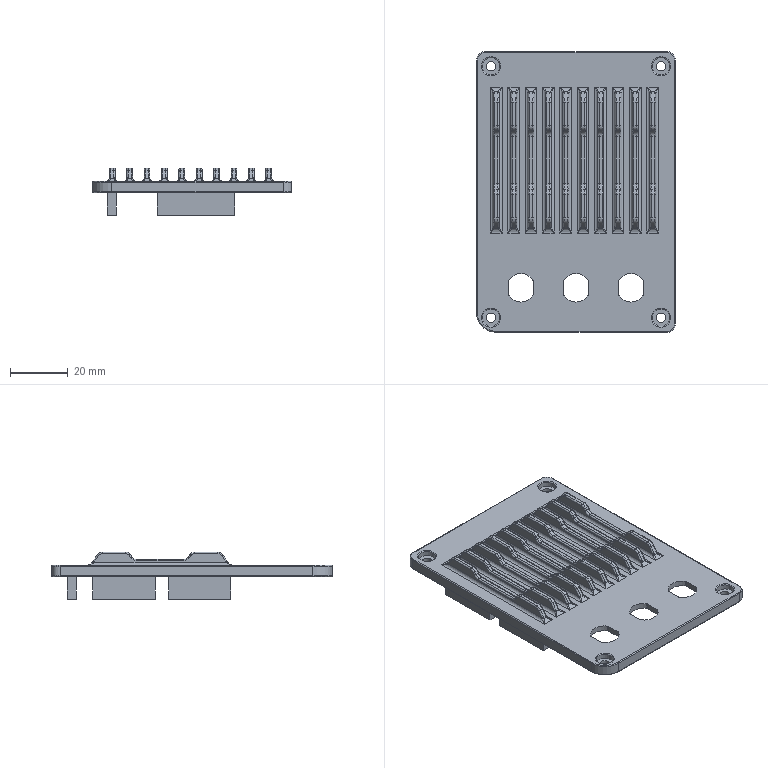NC program | NX | posted with a generic post | part box 68.665 x 96.782 x 16.5 mm
Lines 4650 to 4797 of 111885:
(PLANAR_MILL_COPY_1 , TOOL : 倒角刀)
N9238 T03 M6
N9240 G53
N9242 G17 G0 G90 X-41.991 Y-16.732 S4500 M3
N9244 G43 Z20. H3
N9246 Z2.
N9248 G94 G1 Z-1. F1000.
N9250 G3 X-42.991 Y-15.732 R1.
N9252 G2 X-43.991 Y-14.733 R1.
N9254 G1 X-44.009 Y12.049
N9256 G2 X-43.015 Y13.05 R1.
N9258 G1 X-39.897 Y13.068
N9260 G2 X-38.891 Y12.068 R1.
N9262 G1 Y-14.732
N9264 G2 X-39.891 Y-15.732 R1.
N9266 G1 X-42.991
N9268 G3 X-43.991 Y-16.732 R1.
N9270 G1 Z2.
N9272 G0 Z20.
N9274 X-10.709 Y27.168
N9276 Z2.
N9278 G1 Z-1.
N9280 G3 X-11.709 Y26.168 R1.
N9282 G2 X-12.709 Y25.168 R1.
N9284 G1 X-34.191
N9286 G2 X-35.191 Y26.168 R1.
N9288 G1 Y29.286
N9290 G2 X-34.191 Y30.286 R1.
N9292 G1 X-12.709
N9294 G2 X-11.709 Y29.286 R1.
N9296 G1 Y26.168
N9298 G3 X-10.709 Y25.168 R1.
N9300 G1 Z2.
N9302 G0 Z20.
N9304 X15.409 Y27.168
N9306 Z2.
N9308 G1 Z-1.
N9310 G3 X14.409 Y26.168 R1.
N9312 G2 X13.409 Y25.168 R1.
N9314 G1 X-8.073
N9316 G2 X-9.073 Y26.168 R1.
N9318 G1 Y29.286
N9320 G2 X-8.073 Y30.286 R1.
N9322 G1 X13.409
N9324 G2 X14.409 Y29.286 R1.
N9326 G1 Y26.168
N9328 G3 X15.409 Y25.168 R1.
N9330 G1 Z2.
N9332 G0 Z20.
(PLANAR_MILL_2_COPY , TOOL : 倒角刀)
N9334 X-43.541 Y-37.233
N9336 Z-6.
N9338 G1 Z-9.
N9340 G3 X-45.541 Y-35.233 R2.
N9342 G2 X-49.291 Y-31.483 R3.75
N9344 G1 Y31.483
N9346 G2 X-45.541 Y35.233 R3.75
N9348 G1 X41.741
N9350 G2 X49.291 Y27.683 R7.55
N9352 G1 Y-31.483
N9354 G2 X45.541 Y-35.233 R3.75
N9356 G1 X-45.541
N9358 G3 X-47.541 Y-37.233 R2.
N9360 G1 Z-6.
N9362 G0 Z20.
(PLANAR_MILL_6 , TOOL : 倒角刀)
N9364 X0. Y-30.083
N9366 Z-6.
N9368 G1 Z-9.
N9370 Y-31.583
N9372 X36.976
N9374 G3 X37.656 Y-30.718 R0.7
N9376 G2 X44.777 Y-23.598 R5.9
N9378 G3 X45.641 Y-22.917 R0.7
N9380 G1 Y22.917
N9382 G3 X44.777 Y23.598 R0.7
N9384 G2 X37.656 Y30.718 R5.9
N9386 G3 X36.976 Y31.583 R0.7
N9388 G1 X-36.976
N9390 G3 X-37.656 Y30.718 R0.7
N9392 G2 X-44.777 Y23.598 R5.9
N9394 G3 X-45.641 Y22.917 R0.7
N9396 G1 Y-22.917
N9398 G3 X-44.777 Y-23.598 R0.7
N9400 G2 X-37.656 Y-30.718 R5.9
N9402 G3 X-36.976 Y-31.583 R0.7
N9404 G1 X0.
N9406 Y-30.083
N9408 Z-6.
N9410 G0 Z20.
(PLANAR_MILL_7 , TOOL : 倒角刀)
N9412 X34.069 Y21.373
N9414 Z-8.
N9416 G1 Z-11.
N9418 G3 X33.069 Y22.373 R1.
N9420 G1 X30.824
N9422 X30.767 Y22.355
N9424 G3 X30.767 Y15.691 R4.05
N9426 G1 X30.824 Y15.673
N9428 X35.314
N9430 X35.37 Y15.691
N9432 G3 X35.37 Y22.355 R4.05
N9434 G1 X35.314 Y22.373
N9436 X33.069
N9438 G3 X32.069 Y21.373 R1.
N9440 G1 Z-8.
N9442 G0 Z20.
N9444 X34.069 Y2.373
N9446 Z-8.
N9448 G1 Z-11.
N9450 G3 X33.069 Y3.373 R1.
N9452 G1 X30.824
N9454 X30.767 Y3.355
N9456 G3 X30.767 Y-3.309 R4.05
N9458 G1 X30.824 Y-3.327
N9460 X35.314
N9462 X35.37 Y-3.309
N9464 G3 X35.37 Y3.355 R4.05
N9466 G1 X35.314 Y3.373
N9468 X33.069
N9470 G3 X32.069 Y2.373 R1.
N9472 G1 Z-8.
N9474 G0 Z20.
N9476 Y-21.327
N9478 Z-8.
N9480 G1 Z-11.
N9482 G3 X33.069 Y-22.327 R1.
N9484 G1 X35.314
N9486 X35.37 Y-22.309
N9488 G3 X35.37 Y-15.645 R4.05
N9490 G1 X35.314 Y-15.627
N9492 X30.824
N9494 X30.767 Y-15.645
N9496 G3 X30.767 Y-22.309 R4.05
N9498 G1 X30.824 Y-22.327
N9500 X33.069
N9502 G3 X34.069 Y-21.327 R1.
N9504 G1 Z-8.
N9506 G0 Z20.
N9508 M5